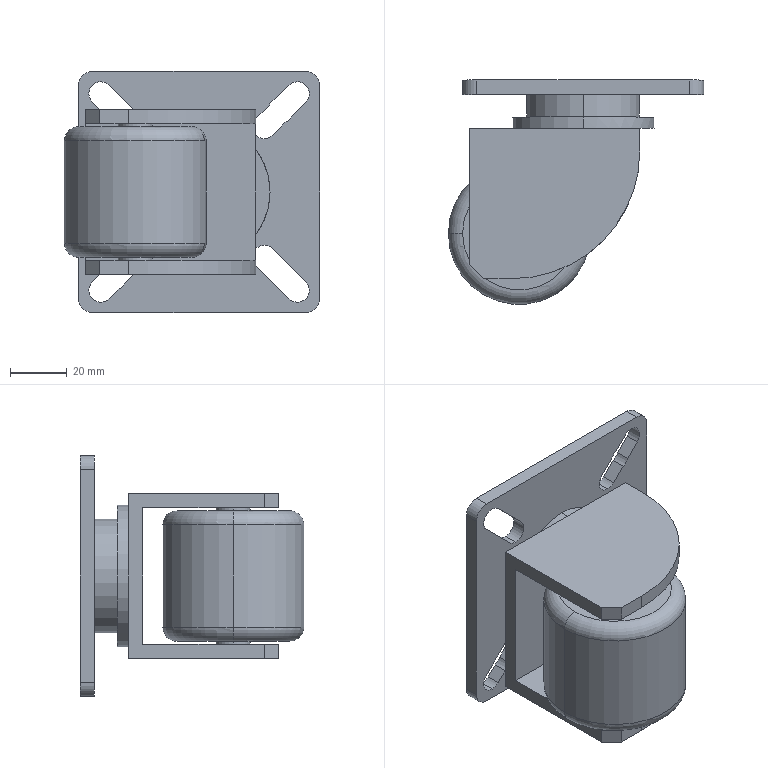Part | STEP file | Medium 2-inch swivel caster J38NZN050R | 1 solid | 84 faces | box 90 x 79 x 85 mm | volume 121466 mm3 | cylinder 38 | plane 38 | torus 8 | commonest cylinder face diameters 8.4 x12 5.6 x4 9 x4 10 x4 12 x4 50 x4